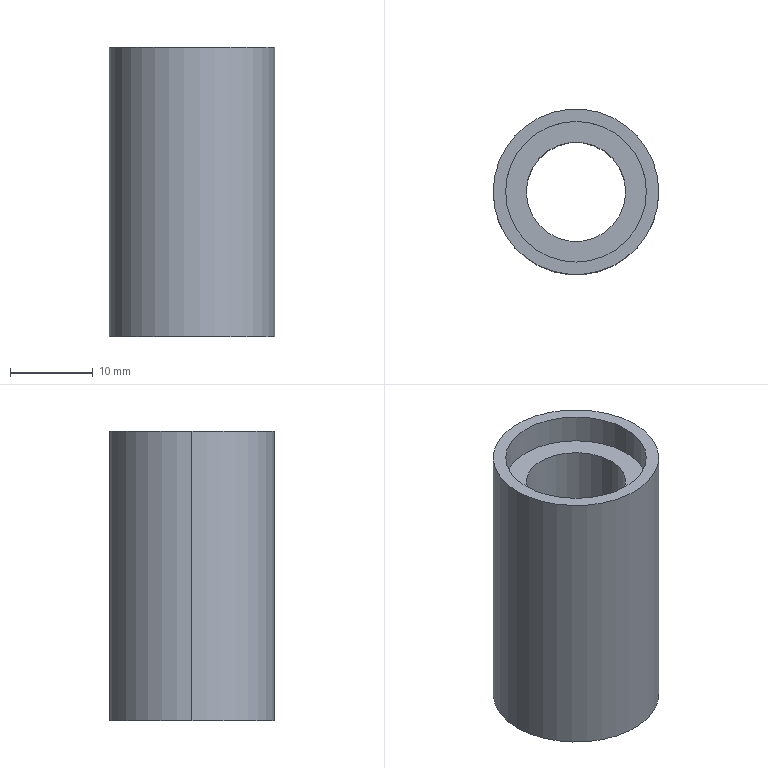Part | STEP file | 1 solid | 11 faces | box 20 x 20 x 35 mm | volume 6555 mm3 | cylinder 6 | plane 3 | cone 2 | commonest cylinder face diameters 12 x2 17 x2 20 x2
STEP:
#1=CARTESIAN_POINT('',(0.,0.,0.));
#2=DIRECTION('',(0.,0.,1.));
#3=DIRECTION('',(1.,0.,0.));
#4=AXIS2_PLACEMENT_3D('',#1,#2,#3);
#5=CARTESIAN_POINT('',(10.,0.,0.));
#6=VERTEX_POINT('',#5);
#7=CARTESIAN_POINT('',(-10.,0.,0.));
#8=VERTEX_POINT('',#7);
#9=CARTESIAN_POINT('',(0.,0.,0.));
#10=DIRECTION('',(0.,0.,1.));
#11=DIRECTION('',(1.,0.,0.));
#12=AXIS2_PLACEMENT_3D('',#9,#10,#11);
#13=CIRCLE('',#12,10.);
#14=CARTESIAN_POINT('',(0.,0.,0.));
#15=DIRECTION('',(0.,0.,1.));
#16=DIRECTION('',(1.,0.,0.));
#17=AXIS2_PLACEMENT_3D('',#14,#15,#16);
#18=CYLINDRICAL_SURFACE('',#17,10.);
#19=CARTESIAN_POINT('',(0.,0.));
#20=DIRECTION('',(1.,0.));
#21=VECTOR('',#20,1.);
#22=LINE('',#19,#21);
#23=(GEOMETRIC_REPRESENTATION_CONTEXT(2)PARAMETRIC_REPRESENTATION_CONTEXT()REPRESENTATION_CONTEXT('',''));
#24=DEFINITIONAL_REPRESENTATION('',(#22),#23);
#25=PCURVE('',#18,#24);
#26=CARTESIAN_POINT('',(0.,0.,0.));
#27=DIRECTION('',(0.,0.,-1.));
#28=DIRECTION('',(-1.,0.,0.));
#29=AXIS2_PLACEMENT_3D('',#26,#27,#28);
#30=PLANE('',#29);
#31=CARTESIAN_POINT('',(-10.,0.));
#32=CARTESIAN_POINT('',(-10.,17.321));
#33=CARTESIAN_POINT('',(5.,8.66));
#34=CARTESIAN_POINT('',(20.,0.));
#35=CARTESIAN_POINT('',(5.,-8.66));
#36=CARTESIAN_POINT('',(-10.,-17.321));
#37=CARTESIAN_POINT('',(-10.,0.));
#38=(BOUNDED_CURVE()B_SPLINE_CURVE(2,(#31,#32,#33,#34,#35,#36,#37),.UNSPECIFIED.,.T.,.F.)B_SPLINE_CURVE_WITH_KNOTS((1,2,2,2,2,1),(-2.094,0.,2.094,4.189,6.283,8.378),.UNSPECIFIED.)CURVE()GEOMETRIC_REPRESENTATION_ITEM()RATIONAL_B_SPLINE_CURVE((1.,0.5,1.,0.5,1.,0.5,1.))REPRESENTATION_ITEM(''));
#39=(GEOMETRIC_REPRESENTATION_CONTEXT(2)PARAMETRIC_REPRESENTATION_CONTEXT()REPRESENTATION_CONTEXT('',''));
#40=DEFINITIONAL_REPRESENTATION('',(#38),#39);
#41=PCURVE('',#30,#40);
#42=SURFACE_CURVE('',#13,(#25,#41),.PCURVE_S1.);
#43=EDGE_CURVE('',#6,#8,#42,.T.);
#44=ORIENTED_EDGE('',*,*,#43,.T.);
#45=CARTESIAN_POINT('',(-10.,0.,35.));
#46=VERTEX_POINT('',#45);
#47=CARTESIAN_POINT('',(-10.,0.,0.));
#48=DIRECTION('',(0.,0.,1.));
#49=VECTOR('',#48,1.);
#50=LINE('',#47,#49);
#51=CARTESIAN_POINT('',(3.142,0.));
#52=DIRECTION('',(0.,1.));
#53=VECTOR('',#52,1.);
#54=LINE('',#51,#53);
#55=(GEOMETRIC_REPRESENTATION_CONTEXT(2)PARAMETRIC_REPRESENTATION_CONTEXT()REPRESENTATION_CONTEXT('',''));
#56=DEFINITIONAL_REPRESENTATION('',(#54),#55);
#57=PCURVE('',#18,#56);
#58=CARTESIAN_POINT('',(0.,0.,0.));
#59=DIRECTION('',(0.,0.,1.));
#60=DIRECTION('',(1.,0.,0.));
#61=AXIS2_PLACEMENT_3D('',#58,#59,#60);
#62=CYLINDRICAL_SURFACE('',#61,10.);
#63=CARTESIAN_POINT('',(3.142,0.));
#64=DIRECTION('',(0.,1.));
#65=VECTOR('',#64,1.);
#66=LINE('',#63,#65);
#67=(GEOMETRIC_REPRESENTATION_CONTEXT(2)PARAMETRIC_REPRESENTATION_CONTEXT()REPRESENTATION_CONTEXT('',''));
#68=DEFINITIONAL_REPRESENTATION('',(#66),#67);
#69=PCURVE('',#62,#68);
#70=SURFACE_CURVE('',#50,(#57,#69),.PCURVE_S1.);
#71=EDGE_CURVE('',#8,#46,#70,.T.);
#72=ORIENTED_EDGE('',*,*,#71,.T.);
#73=CARTESIAN_POINT('',(10.,0.,35.));
#74=VERTEX_POINT('',#73);
#75=CARTESIAN_POINT('',(0.,0.,35.));
#76=DIRECTION('',(0.,0.,-1.));
#77=DIRECTION('',(1.,0.,0.));
#78=AXIS2_PLACEMENT_3D('',#75,#76,#77);
#79=CIRCLE('',#78,10.);
#80=CARTESIAN_POINT('',(6.283,35.));
#81=DIRECTION('',(-1.,0.));
#82=VECTOR('',#81,1.);
#83=LINE('',#80,#82);
#84=(GEOMETRIC_REPRESENTATION_CONTEXT(2)PARAMETRIC_REPRESENTATION_CONTEXT()REPRESENTATION_CONTEXT('',''));
#85=DEFINITIONAL_REPRESENTATION('',(#83),#84);
#86=PCURVE('',#18,#85);
#87=CARTESIAN_POINT('',(0.,0.,35.));
#88=DIRECTION('',(0.,0.,-1.));
#89=DIRECTION('',(-1.,0.,0.));
#90=AXIS2_PLACEMENT_3D('',#87,#88,#89);
#91=PLANE('',#90);
#92=CARTESIAN_POINT('',(0.,0.));
#93=DIRECTION('',(-1.,0.));
#94=AXIS2_PLACEMENT_2D('',#92,#93);
#95=CIRCLE('',#94,10.);
#96=(GEOMETRIC_REPRESENTATION_CONTEXT(2)PARAMETRIC_REPRESENTATION_CONTEXT()REPRESENTATION_CONTEXT('',''));
#97=DEFINITIONAL_REPRESENTATION('',(#95),#96);
#98=PCURVE('',#91,#97);
#99=SURFACE_CURVE('',#79,(#86,#98),.PCURVE_S1.);
#100=EDGE_CURVE('',#46,#74,#99,.T.);
#101=ORIENTED_EDGE('',*,*,#100,.T.);
#102=CARTESIAN_POINT('',(10.,0.,0.));
#103=DIRECTION('',(0.,0.,1.));
#104=VECTOR('',#103,1.);
#105=LINE('',#102,#104);
#106=CARTESIAN_POINT('',(0.,0.));
#107=DIRECTION('',(0.,1.));
#108=VECTOR('',#107,1.);
#109=LINE('',#106,#108);
#110=(GEOMETRIC_REPRESENTATION_CONTEXT(2)PARAMETRIC_REPRESENTATION_CONTEXT()REPRESENTATION_CONTEXT('',''));
#111=DEFINITIONAL_REPRESENTATION('',(#109),#110);
#112=PCURVE('',#18,#111);
#113=CARTESIAN_POINT('',(6.283,0.));
#114=DIRECTION('',(0.,1.));
#115=VECTOR('',#114,1.);
#116=LINE('',#113,#115);
#117=(GEOMETRIC_REPRESENTATION_CONTEXT(2)PARAMETRIC_REPRESENTATION_CONTEXT()REPRESENTATION_CONTEXT('',''));
#118=DEFINITIONAL_REPRESENTATION('',(#116),#117);
#119=PCURVE('',#62,#118);
#120=SURFACE_CURVE('',#105,(#112,#119),.PCURVE_S1.);
#121=EDGE_CURVE('',#6,#74,#120,.T.);
#122=ORIENTED_EDGE('',*,*,#121,.F.);
#123=EDGE_LOOP('',(#44,#72,#101,#122));
#124=FACE_BOUND('',#123,.T.);
#125=ADVANCED_FACE('',(#124),#18,.T.);
#126=CARTESIAN_POINT('',(-6.,0.,2.));
#127=VERTEX_POINT('',#126);
#128=CARTESIAN_POINT('',(-8.,0.,-0.000000001));
#129=VERTEX_POINT('',#128);
#130=CARTESIAN_POINT('',(-8.,0.,-0.000000001));
#131=DIRECTION('',(-0.7071,0.,-0.7071));
#132=VECTOR('',#131,1.);
#133=LINE('',#130,#132);
#134=CARTESIAN_POINT('',(0.,0.,-0.000000001));
#135=DIRECTION('',(0.,0.,-1.));
#136=DIRECTION('',(-1.,0.,0.));
#137=AXIS2_PLACEMENT_3D('',#134,#135,#136);
#138=CONICAL_SURFACE('',#137,8.,0.7854);
#139=CARTESIAN_POINT('',(6.283,0.));
#140=DIRECTION('',(0.,1.));
#141=VECTOR('',#140,1.);
#142=LINE('',#139,#141);
#143=(GEOMETRIC_REPRESENTATION_CONTEXT(2)PARAMETRIC_REPRESENTATION_CONTEXT()REPRESENTATION_CONTEXT('',''));
#144=DEFINITIONAL_REPRESENTATION('',(#142),#143);
#145=PCURVE('',#138,#144);
#146=CARTESIAN_POINT('',(0.,0.,-0.000000001));
#147=DIRECTION('',(0.,0.,-1.));
#148=DIRECTION('',(-1.,0.,0.));
#149=AXIS2_PLACEMENT_3D('',#146,#147,#148);
#150=CONICAL_SURFACE('',#149,8.,0.7854);
#151=CARTESIAN_POINT('',(0.,0.));
#152=DIRECTION('',(0.,1.));
#153=VECTOR('',#152,1.);
#154=LINE('',#151,#153);
#155=(GEOMETRIC_REPRESENTATION_CONTEXT(2)PARAMETRIC_REPRESENTATION_CONTEXT()REPRESENTATION_CONTEXT('',''));
#156=DEFINITIONAL_REPRESENTATION('',(#154),#155);
#157=PCURVE('',#150,#156);
#158=SURFACE_CURVE('',#133,(#145,#157),.PCURVE_S1.);
#159=EDGE_CURVE('',#127,#129,#158,.T.);
#160=ORIENTED_EDGE('',*,*,#159,.T.);
#161=CARTESIAN_POINT('',(8.,0.,-0.000000001));
#162=VERTEX_POINT('',#161);
#163=CARTESIAN_POINT('',(0.,0.,-0.000000001));
#164=DIRECTION('',(0.,0.,1.));
#165=DIRECTION('',(-1.,0.,0.));
#166=AXIS2_PLACEMENT_3D('',#163,#164,#165);
#167=CIRCLE('',#166,8.);
#168=CARTESIAN_POINT('',(6.283,0.));
#169=DIRECTION('',(-1.,0.));
#170=VECTOR('',#169,1.);
#171=LINE('',#168,#170);
#172=(GEOMETRIC_REPRESENTATION_CONTEXT(2)PARAMETRIC_REPRESENTATION_CONTEXT()REPRESENTATION_CONTEXT('',''));
#173=DEFINITIONAL_REPRESENTATION('',(#171),#172);
#174=PCURVE('',#138,#173);
#175=CARTESIAN_POINT('',(8.,0.));
#176=CARTESIAN_POINT('',(8.,-13.856));
#177=CARTESIAN_POINT('',(-4.,-6.928));
#178=CARTESIAN_POINT('',(-16.,0.));
#179=CARTESIAN_POINT('',(-4.,6.928));
#180=CARTESIAN_POINT('',(8.,13.856));
#181=CARTESIAN_POINT('',(8.,0.));
#182=(BOUNDED_CURVE()B_SPLINE_CURVE(2,(#175,#176,#177,#178,#179,#180,#181),.UNSPECIFIED.,.T.,.F.)B_SPLINE_CURVE_WITH_KNOTS((1,2,2,2,2,1),(-2.094,0.,2.094,4.189,6.283,8.378),.UNSPECIFIED.)CURVE()GEOMETRIC_REPRESENTATION_ITEM()RATIONAL_B_SPLINE_CURVE((1.,0.5,1.,0.5,1.,0.5,1.))REPRESENTATION_ITEM(''));
#183=(GEOMETRIC_REPRESENTATION_CONTEXT(2)PARAMETRIC_REPRESENTATION_CONTEXT()REPRESENTATION_CONTEXT('',''));
#184=DEFINITIONAL_REPRESENTATION('',(#182),#183);
#185=PCURVE('',#30,#184);
#186=SURFACE_CURVE('',#167,(#174,#185),.PCURVE_S1.);
#187=EDGE_CURVE('',#129,#162,#186,.T.);
#188=ORIENTED_EDGE('',*,*,#187,.T.);
#189=CARTESIAN_POINT('',(6.,0.,2.));
#190=VERTEX_POINT('',#189);
#191=CARTESIAN_POINT('',(8.,0.,-0.000000001));
#192=DIRECTION('',(0.7071,0.,-0.7071));
#193=VECTOR('',#192,1.);
#194=LINE('',#191,#193);
#195=CARTESIAN_POINT('',(3.142,0.));
#196=DIRECTION('',(0.,1.));
#197=VECTOR('',#196,1.);
#198=LINE('',#195,#197);
#199=(GEOMETRIC_REPRESENTATION_CONTEXT(2)PARAMETRIC_REPRESENTATION_CONTEXT()REPRESENTATION_CONTEXT('',''));
#200=DEFINITIONAL_REPRESENTATION('',(#198),#199);
#201=PCURVE('',#138,#200);
#202=CARTESIAN_POINT('',(3.142,0.));
#203=DIRECTION('',(0.,1.));
#204=VECTOR('',#203,1.);
#205=LINE('',#202,#204);
#206=(GEOMETRIC_REPRESENTATION_CONTEXT(2)PARAMETRIC_REPRESENTATION_CONTEXT()REPRESENTATION_CONTEXT('',''));
#207=DEFINITIONAL_REPRESENTATION('',(#205),#206);
#208=PCURVE('',#150,#207);
#209=SURFACE_CURVE('',#194,(#201,#208),.PCURVE_S1.);
#210=EDGE_CURVE('',#190,#162,#209,.T.);
#211=ORIENTED_EDGE('',*,*,#210,.F.);
#212=CARTESIAN_POINT('',(0.,0.,2.));
#213=DIRECTION('',(0.,0.,-1.));
#214=DIRECTION('',(1.,0.,0.));
#215=AXIS2_PLACEMENT_3D('',#212,#213,#214);
#216=CIRCLE('',#215,6.);
#217=CARTESIAN_POINT('',(3.142,-2.));
#218=DIRECTION('',(1.,0.));
#219=VECTOR('',#218,1.);
#220=LINE('',#217,#219);
#221=(GEOMETRIC_REPRESENTATION_CONTEXT(2)PARAMETRIC_REPRESENTATION_CONTEXT()REPRESENTATION_CONTEXT('',''));
#222=DEFINITIONAL_REPRESENTATION('',(#220),#221);
#223=PCURVE('',#138,#222);
#224=CARTESIAN_POINT('',(0.,0.,0.));
#225=DIRECTION('',(0.,0.,1.));
#226=DIRECTION('',(1.,0.,0.));
#227=AXIS2_PLACEMENT_3D('',#224,#225,#226);
#228=CYLINDRICAL_SURFACE('',#227,6.);
#229=CARTESIAN_POINT('',(6.283,2.));
#230=DIRECTION('',(-1.,0.));
#231=VECTOR('',#230,1.);
#232=LINE('',#229,#231);
#233=(GEOMETRIC_REPRESENTATION_CONTEXT(2)PARAMETRIC_REPRESENTATION_CONTEXT()REPRESENTATION_CONTEXT('',''));
#234=DEFINITIONAL_REPRESENTATION('',(#232),#233);
#235=PCURVE('',#228,#234);
#236=SURFACE_CURVE('',#216,(#223,#235),.PCURVE_S1.);
#237=EDGE_CURVE('',#190,#127,#236,.T.);
#238=ORIENTED_EDGE('',*,*,#237,.T.);
#239=EDGE_LOOP('',(#160,#188,#211,#238));
#240=FACE_BOUND('',#239,.F.);
#241=ADVANCED_FACE('',(#240),#138,.F.);
#242=CARTESIAN_POINT('',(-8.5,0.,35.));
#243=VERTEX_POINT('',#242);
#244=CARTESIAN_POINT('',(-8.5,0.,31.5));
#245=VERTEX_POINT('',#244);
#246=CARTESIAN_POINT('',(-8.5,0.,35.));
#247=DIRECTION('',(0.,0.,-1.));
#248=VECTOR('',#247,1.);
#249=LINE('',#246,#248);
#250=CARTESIAN_POINT('',(0.,0.,35.));
#251=DIRECTION('',(0.,0.,-1.));
#252=DIRECTION('',(-1.,0.,0.));
#253=AXIS2_PLACEMENT_3D('',#250,#251,#252);
#254=CYLINDRICAL_SURFACE('',#253,8.5);
#255=CARTESIAN_POINT('',(6.283,0.));
#256=DIRECTION('',(0.,1.));
#257=VECTOR('',#256,1.);
#258=LINE('',#255,#257);
#259=(GEOMETRIC_REPRESENTATION_CONTEXT(2)PARAMETRIC_REPRESENTATION_CONTEXT()REPRESENTATION_CONTEXT('',''));
#260=DEFINITIONAL_REPRESENTATION('',(#258),#259);
#261=PCURVE('',#254,#260);
#262=CARTESIAN_POINT('',(0.,0.,35.));
#263=DIRECTION('',(0.,0.,-1.));
#264=DIRECTION('',(-1.,0.,0.));
#265=AXIS2_PLACEMENT_3D('',#262,#263,#264);
#266=CYLINDRICAL_SURFACE('',#265,8.5);
#267=CARTESIAN_POINT('',(0.,0.));
#268=DIRECTION('',(0.,1.));
#269=VECTOR('',#268,1.);
#270=LINE('',#267,#269);
#271=(GEOMETRIC_REPRESENTATION_CONTEXT(2)PARAMETRIC_REPRESENTATION_CONTEXT()REPRESENTATION_CONTEXT('',''));
#272=DEFINITIONAL_REPRESENTATION('',(#270),#271);
#273=PCURVE('',#266,#272);
#274=SURFACE_CURVE('',#249,(#261,#273),.PCURVE_S1.);
#275=EDGE_CURVE('',#243,#245,#274,.T.);
#276=ORIENTED_EDGE('',*,*,#275,.T.);
#277=CARTESIAN_POINT('',(8.5,0.,31.5));
#278=VERTEX_POINT('',#277);
#279=CARTESIAN_POINT('',(0.,0.,31.5));
#280=DIRECTION('',(0.,0.,1.));
#281=DIRECTION('',(-1.,0.,0.));
#282=AXIS2_PLACEMENT_3D('',#279,#280,#281);
#283=CIRCLE('',#282,8.5);
#284=CARTESIAN_POINT('',(6.283,3.5));
#285=DIRECTION('',(-1.,0.));
#286=VECTOR('',#285,1.);
#287=LINE('',#284,#286);
#288=(GEOMETRIC_REPRESENTATION_CONTEXT(2)PARAMETRIC_REPRESENTATION_CONTEXT()REPRESENTATION_CONTEXT('',''));
#289=DEFINITIONAL_REPRESENTATION('',(#287),#288);
#290=PCURVE('',#254,#289);
#291=CARTESIAN_POINT('',(0.,0.,31.5));
#292=DIRECTION('',(0.,0.,-1.));
#293=DIRECTION('',(-1.,0.,0.));
#294=AXIS2_PLACEMENT_3D('',#291,#292,#293);
#295=PLANE('',#294);
#296=CARTESIAN_POINT('',(8.5,0.));
#297=CARTESIAN_POINT('',(8.5,-14.722));
#298=CARTESIAN_POINT('',(-4.25,-7.361));
#299=CARTESIAN_POINT('',(-17.,0.));
#300=CARTESIAN_POINT('',(-4.25,7.361));
#301=CARTESIAN_POINT('',(8.5,14.722));
#302=CARTESIAN_POINT('',(8.5,0.));
#303=(BOUNDED_CURVE()B_SPLINE_CURVE(2,(#296,#297,#298,#299,#300,#301,#302),.UNSPECIFIED.,.T.,.F.)B_SPLINE_CURVE_WITH_KNOTS((1,2,2,2,2,1),(-2.094,0.,2.094,4.189,6.283,8.378),.UNSPECIFIED.)CURVE()GEOMETRIC_REPRESENTATION_ITEM()RATIONAL_B_SPLINE_CURVE((1.,0.5,1.,0.5,1.,0.5,1.))REPRESENTATION_ITEM(''));
#304=(GEOMETRIC_REPRESENTATION_CONTEXT(2)PARAMETRIC_REPRESENTATION_CONTEXT()REPRESENTATION_CONTEXT('',''));
#305=DEFINITIONAL_REPRESENTATION('',(#303),#304);
#306=PCURVE('',#295,#305);
#307=SURFACE_CURVE('',#283,(#290,#306),.PCURVE_S1.);
#308=EDGE_CURVE('',#245,#278,#307,.T.);
#309=ORIENTED_EDGE('',*,*,#308,.T.);
#310=CARTESIAN_POINT('',(8.5,0.,35.));
#311=VERTEX_POINT('',#310);
#312=CARTESIAN_POINT('',(8.5,0.,35.));
#313=DIRECTION('',(0.,0.,-1.));
#314=VECTOR('',#313,1.);
#315=LINE('',#312,#314);
#316=CARTESIAN_POINT('',(3.142,0.));
#317=DIRECTION('',(0.,1.));
#318=VECTOR('',#317,1.);
#319=LINE('',#316,#318);
#320=(GEOMETRIC_REPRESENTATION_CONTEXT(2)PARAMETRIC_REPRESENTATION_CONTEXT()REPRESENTATION_CONTEXT('',''));
#321=DEFINITIONAL_REPRESENTATION('',(#319),#320);
#322=PCURVE('',#254,#321);
#323=CARTESIAN_POINT('',(3.142,0.));
#324=DIRECTION('',(0.,1.));
#325=VECTOR('',#324,1.);
#326=LINE('',#323,#325);
#327=(GEOMETRIC_REPRESENTATION_CONTEXT(2)PARAMETRIC_REPRESENTATION_CONTEXT()REPRESENTATION_CONTEXT('',''));
#328=DEFINITIONAL_REPRESENTATION('',(#326),#327);
#329=PCURVE('',#266,#328);
#330=SURFACE_CURVE('',#315,(#322,#329),.PCURVE_S1.);
#331=EDGE_CURVE('',#311,#278,#330,.T.);
#332=ORIENTED_EDGE('',*,*,#331,.F.);
#333=CARTESIAN_POINT('',(0.,0.,35.));
#334=DIRECTION('',(0.,0.,1.));
#335=DIRECTION('',(-1.,0.,0.));
#336=AXIS2_PLACEMENT_3D('',#333,#334,#335);
#337=CIRCLE('',#336,8.5);
#338=CARTESIAN_POINT('',(6.283,0.));
#339=DIRECTION('',(-1.,0.));
#340=VECTOR('',#339,1.);
#341=LINE('',#338,#340);
#342=(GEOMETRIC_REPRESENTATION_CONTEXT(2)PARAMETRIC_REPRESENTATION_CONTEXT()REPRESENTATION_CONTEXT('',''));
#343=DEFINITIONAL_REPRESENTATION('',(#341),#342);
#344=PCURVE('',#254,#343);
#345=CARTESIAN_POINT('',(8.5,0.));
#346=CARTESIAN_POINT('',(8.5,-14.722));
#347=CARTESIAN_POINT('',(-4.25,-7.361));
#348=CARTESIAN_POINT('',(-17.,0.));
#349=CARTESIAN_POINT('',(-4.25,7.361));
#350=CARTESIAN_POINT('',(8.5,14.722));
#351=CARTESIAN_POINT('',(8.5,0.));
#352=(BOUNDED_CURVE()B_SPLINE_CURVE(2,(#345,#346,#347,#348,#349,#350,#351),.UNSPECIFIED.,.T.,.F.)B_SPLINE_CURVE_WITH_KNOTS((1,2,2,2,2,1),(-2.094,0.,2.094,4.189,6.283,8.378),.UNSPECIFIED.)CURVE()GEOMETRIC_REPRESENTATION_ITEM()RATIONAL_B_SPLINE_CURVE((1.,0.5,1.,0.5,1.,0.5,1.))REPRESENTATION_ITEM(''));
#353=(GEOMETRIC_REPRESENTATION_CONTEXT(2)PARAMETRIC_REPRESENTATION_CONTEXT()REPRESENTATION_CONTEXT('',''));
#354=DEFINITIONAL_REPRESENTATION('',(#352),#353);
#355=PCURVE('',#91,#354);
#356=SURFACE_CURVE('',#337,(#344,#355),.PCURVE_S1.);
#357=EDGE_CURVE('',#243,#311,#356,.T.);
#358=ORIENTED_EDGE('',*,*,#357,.F.);
#359=EDGE_LOOP('',(#276,#309,#332,#358));
#360=FACE_BOUND('',#359,.F.);
#361=ADVANCED_FACE('',(#360),#254,.F.);
#362=CARTESIAN_POINT('',(6.,0.,31.5));
#363=VERTEX_POINT('',#362);
#364=CARTESIAN_POINT('',(6.,0.,0.));
#365=DIRECTION('',(0.,0.,1.));
#366=VECTOR('',#365,1.);
#367=LINE('',#364,#366);
#368=CARTESIAN_POINT('',(6.283,0.));
#369=DIRECTION('',(0.,1.));
#370=VECTOR('',#369,1.);
#371=LINE('',#368,#370);
#372=(GEOMETRIC_REPRESENTATION_CONTEXT(2)PARAMETRIC_REPRESENTATION_CONTEXT()REPRESENTATION_CONTEXT('',''));
#373=DEFINITIONAL_REPRESENTATION('',(#371),#372);
#374=PCURVE('',#228,#373);
#375=CARTESIAN_POINT('',(0.,0.,0.));
#376=DIRECTION('',(0.,0.,1.));
#377=DIRECTION('',(1.,0.,0.));
#378=AXIS2_PLACEMENT_3D('',#375,#376,#377);
#379=CYLINDRICAL_SURFACE('',#378,6.);
#380=CARTESIAN_POINT('',(0.,0.));
#381=DIRECTION('',(0.,1.));
#382=VECTOR('',#381,1.);
#383=LINE('',#380,#382);
#384=(GEOMETRIC_REPRESENTATION_CONTEXT(2)PARAMETRIC_REPRESENTATION_CONTEXT()REPRESENTATION_CONTEXT('',''));
#385=DEFINITIONAL_REPRESENTATION('',(#383),#384);
#386=PCURVE('',#379,#385);
#387=SURFACE_CURVE('',#367,(#374,#386),.PCURVE_S1.);
#388=EDGE_CURVE('',#190,#363,#387,.T.);
#389=ORIENTED_EDGE('',*,*,#388,.T.);
#390=CARTESIAN_POINT('',(-6.,0.,31.5));
#391=VERTEX_POINT('',#390);
#392=CARTESIAN_POINT('',(0.,0.,31.5));
#393=DIRECTION('',(0.,0.,-1.));
#394=DIRECTION('',(1.,0.,0.));
#395=AXIS2_PLACEMENT_3D('',#392,#393,#394);
#396=CIRCLE('',#395,6.);
#397=CARTESIAN_POINT('',(6.283,31.5));
#398=DIRECTION('',(-1.,0.));
#399=VECTOR('',#398,1.);
#400=LINE('',#397,#399);
#401=(GEOMETRIC_REPRESENTATION_CONTEXT(2)PARAMETRIC_REPRESENTATION_CONTEXT()REPRESENTATION_CONTEXT('',''));
#402=DEFINITIONAL_REPRESENTATION('',(#400),#401);
#403=PCURVE('',#228,#402);
#404=CARTESIAN_POINT('',(0.,0.));
#405=DIRECTION('',(-1.,0.));
#406=AXIS2_PLACEMENT_2D('',#404,#405);
#407=CIRCLE('',#406,6.);
#408=(GEOMETRIC_REPRESENTATION_CONTEXT(2)PARAMETRIC_REPRESENTATION_CONTEXT()REPRESENTATION_CONTEXT('',''));
#409=DEFINITIONAL_REPRESENTATION('',(#407),#408);
#410=PCURVE('',#295,#409);
#411=SURFACE_CURVE('',#396,(#403,#410),.PCURVE_S1.);
#412=EDGE_CURVE('',#363,#391,#411,.T.);
#413=ORIENTED_EDGE('',*,*,#412,.T.);
#414=CARTESIAN_POINT('',(-6.,0.,0.));
#415=DIRECTION('',(0.,0.,1.));
#416=VECTOR('',#415,1.);
#417=LINE('',#414,#416);
#418=CARTESIAN_POINT('',(3.142,0.));
#419=DIRECTION('',(0.,1.));
#420=VECTOR('',#419,1.);
#421=LINE('',#418,#420);
#422=(GEOMETRIC_REPRESENTATION_CONTEXT(2)PARAMETRIC_REPRESENTATION_CONTEXT()REPRESENTATION_CONTEXT('',''));
#423=DEFINITIONAL_REPRESENTATION('',(#421),#422);
#424=PCURVE('',#228,#423);
#425=CARTESIAN_POINT('',(3.142,0.));
#426=DIRECTION('',(0.,1.));
#427=VECTOR('',#426,1.);
#428=LINE('',#425,#427);
#429=(GEOMETRIC_REPRESENTATION_CONTEXT(2)PARAMETRIC_REPRESENTATION_CONTEXT()REPRESENTATION_CONTEXT('',''));
#430=DEFINITIONAL_REPRESENTATION('',(#428),#429);
#431=PCURVE('',#379,#430);
#432=SURFACE_CURVE('',#417,(#424,#431),.PCURVE_S1.);
#433=EDGE_CURVE('',#127,#391,#432,.T.);
#434=ORIENTED_EDGE('',*,*,#433,.F.);
#435=ORIENTED_EDGE('',*,*,#237,.F.);
#436=EDGE_LOOP('',(#389,#413,#434,#435));
#437=FACE_BOUND('',#436,.F.);
#438=ADVANCED_FACE('',(#437),#228,.F.);
#439=ORIENTED_EDGE('',*,*,#71,.F.);
#440=CARTESIAN_POINT('',(0.,0.,0.));
#441=DIRECTION('',(0.,0.,1.));
#442=DIRECTION('',(1.,0.,0.));
#443=AXIS2_PLACEMENT_3D('',#440,#441,#442);
#444=CIRCLE('',#443,10.);
#445=CARTESIAN_POINT('',(0.,0.));
#446=DIRECTION('',(1.,0.));
#447=VECTOR('',#446,1.);
#448=LINE('',#445,#447);
#449=(GEOMETRIC_REPRESENTATION_CONTEXT(2)PARAMETRIC_REPRESENTATION_CONTEXT()REPRESENTATION_CONTEXT('',''));
#450=DEFINITIONAL_REPRESENTATION('',(#448),#449);
#451=PCURVE('',#62,#450);
#452=CARTESIAN_POINT('',(-10.,0.));
#453=CARTESIAN_POINT('',(-10.,17.321));
#454=CARTESIAN_POINT('',(5.,8.66));
#455=CARTESIAN_POINT('',(20.,0.));
#456=CARTESIAN_POINT('',(5.,-8.66));
#457=CARTESIAN_POINT('',(-10.,-17.321));
#458=CARTESIAN_POINT('',(-10.,0.));
#459=(BOUNDED_CURVE()B_SPLINE_CURVE(2,(#452,#453,#454,#455,#456,#457,#458),.UNSPECIFIED.,.T.,.F.)B_SPLINE_CURVE_WITH_KNOTS((1,2,2,2,2,1),(-2.094,0.,2.094,4.189,6.283,8.378),.UNSPECIFIED.)CURVE()GEOMETRIC_REPRESENTATION_ITEM()RATIONAL_B_SPLINE_CURVE((1.,0.5,1.,0.5,1.,0.5,1.))REPRESENTATION_ITEM(''));
#460=(GEOMETRIC_REPRESENTATION_CONTEXT(2)PARAMETRIC_REPRESENTATION_CONTEXT()REPRESENTATION_CONTEXT('',''));
#461=DEFINITIONAL_REPRESENTATION('',(#459),#460);
#462=PCURVE('',#30,#461);
#463=SURFACE_CURVE('',#444,(#451,#462),.PCURVE_S1.);
#464=EDGE_CURVE('',#8,#6,#463,.T.);
#465=ORIENTED_EDGE('',*,*,#464,.T.);
#466=ORIENTED_EDGE('',*,*,#121,.T.);
#467=CARTESIAN_POINT('',(0.,0.,35.));
#468=DIRECTION('',(0.,0.,-1.));
#469=DIRECTION('',(1.,0.,0.));
#470=AXIS2_PLACEMENT_3D('',#467,#468,#469);
#471=CIRCLE('',#470,10.);
#472=CARTESIAN_POINT('',(6.283,35.));
#473=DIRECTION('',(-1.,0.));
#474=VECTOR('',#473,1.);
#475=LINE('',#472,#474);
#476=(GEOMETRIC_REPRESENTATION_CONTEXT(2)PARAMETRIC_REPRESENTATION_CONTEXT()REPRESENTATION_CONTEXT('',''));
#477=DEFINITIONAL_REPRESENTATION('',(#475),#476);
#478=PCURVE('',#62,#477);
#479=CARTESIAN_POINT('',(0.,0.));
#480=DIRECTION('',(-1.,0.));
#481=AXIS2_PLACEMENT_2D('',#479,#480);
#482=CIRCLE('',#481,10.);
#483=(GEOMETRIC_REPRESENTATION_CONTEXT(2)PARAMETRIC_REPRESENTATION_CONTEXT()REPRESENTATION_CONTEXT('',''));
#484=DEFINITIONAL_REPRESENTATION('',(#482),#483);
#485=PCURVE('',#91,#484);
#486=SURFACE_CURVE('',#471,(#478,#485),.PCURVE_S1.);
#487=EDGE_CURVE('',#74,#46,#486,.T.);
#488=ORIENTED_EDGE('',*,*,#487,.T.);
#489=EDGE_LOOP('',(#439,#465,#466,#488));
#490=FACE_BOUND('',#489,.T.);
#491=ADVANCED_FACE('',(#490),#62,.T.);
#492=ORIENTED_EDGE('',*,*,#187,.T.);
#493=CARTESIAN_POINT('',(0.,0.,-0.000000001));
#494=DIRECTION('',(0.,0.,1.));
#495=DIRECTION('',(-1.,0.,0.));
#496=AXIS2_PLACEMENT_3D('',#493,#494,#495);
#497=CIRCLE('',#496,8.);
#498=CARTESIAN_POINT('',(8.,0.));
#499=CARTESIAN_POINT('',(8.,-13.856));
#500=CARTESIAN_POINT('',(-4.,-6.928));
#501=CARTESIAN_POINT('',(-16.,0.));
#502=CARTESIAN_POINT('',(-4.,6.928));
#503=CARTESIAN_POINT('',(8.,13.856));
#504=CARTESIAN_POINT('',(8.,0.));
#505=(BOUNDED_CURVE()B_SPLINE_CURVE(2,(#498,#499,#500,#501,#502,#503,#504),.UNSPECIFIED.,.T.,.F.)B_SPLINE_CURVE_WITH_KNOTS((1,2,2,2,2,1),(-2.094,0.,2.094,4.189,6.283,8.378),.UNSPECIFIED.)CURVE()GEOMETRIC_REPRESENTATION_ITEM()RATIONAL_B_SPLINE_CURVE((1.,0.5,1.,0.5,1.,0.5,1.))REPRESENTATION_ITEM(''));
#506=(GEOMETRIC_REPRESENTATION_CONTEXT(2)PARAMETRIC_REPRESENTATION_CONTEXT()REPRESENTATION_CONTEXT('',''));
#507=DEFINITIONAL_REPRESENTATION('',(#505),#506);
#508=PCURVE('',#30,#507);
#509=CARTESIAN_POINT('',(6.283,0.));
#510=DIRECTION('',(-1.,0.));
#511=VECTOR('',#510,1.);
#512=LINE('',#509,#511);
#513=(GEOMETRIC_REPRESENTATION_CONTEXT(2)PARAMETRIC_REPRESENTATION_CONTEXT()REPRESENTATION_CONTEXT('',''));
#514=DEFINITIONAL_REPRESENTATION('',(#512),#513);
#515=PCURVE('',#150,#514);
#516=SURFACE_CURVE('',#497,(#508,#515),.PCURVE_S1.);
#517=EDGE_CURVE('',#162,#129,#516,.T.);
#518=ORIENTED_EDGE('',*,*,#517,.T.);
#519=EDGE_LOOP('',(#492,#518));
#520=FACE_BOUND('',#519,.T.);
#521=ORIENTED_EDGE('',*,*,#43,.F.);
#522=ORIENTED_EDGE('',*,*,#464,.F.);
#523=EDGE_LOOP('',(#521,#522));
#524=FACE_BOUND('',#523,.T.);
#525=ADVANCED_FACE('',(#520,#524),#30,.T.);
#526=ORIENTED_EDGE('',*,*,#357,.F.);
#527=CARTESIAN_POINT('',(0.,0.,35.));
#528=DIRECTION('',(0.,0.,1.));
#529=DIRECTION('',(-1.,0.,0.));
#530=AXIS2_PLACEMENT_3D('',#527,#528,#529);
#531=CIRCLE('',#530,8.5);
#532=CARTESIAN_POINT('',(8.5,0.));
#533=CARTESIAN_POINT('',(8.5,-14.722));
#534=CARTESIAN_POINT('',(-4.25,-7.361));
#535=CARTESIAN_POINT('',(-17.,0.));
#536=CARTESIAN_POINT('',(-4.25,7.361));
#537=CARTESIAN_POINT('',(8.5,14.722));
#538=CARTESIAN_POINT('',(8.5,0.));
#539=(BOUNDED_CURVE()B_SPLINE_CURVE(2,(#532,#533,#534,#535,#536,#537,#538),.UNSPECIFIED.,.T.,.F.)B_SPLINE_CURVE_WITH_KNOTS((1,2,2,2,2,1),(-2.094,0.,2.094,4.189,6.283,8.378),.UNSPECIFIED.)CURVE()GEOMETRIC_REPRESENTATION_ITEM()RATIONAL_B_SPLINE_CURVE((1.,0.5,1.,0.5,1.,0.5,1.))REPRESENTATION_ITEM(''));
#540=(GEOMETRIC_REPRESENTATION_CONTEXT(2)PARAMETRIC_REPRESENTATION_CONTEXT()REPRESENTATION_CONTEXT('',''));
#541=DEFINITIONAL_REPRESENTATION('',(#539),#540);
#542=PCURVE('',#91,#541);
#543=CARTESIAN_POINT('',(6.283,0.));
#544=DIRECTION('',(-1.,0.));
#545=VECTOR('',#544,1.);
#546=LINE('',#543,#545);
#547=(GEOMETRIC_REPRESENTATION_CONTEXT(2)PARAMETRIC_REPRESENTATION_CONTEXT()REPRESENTATION_CONTEXT('',''));
#548=DEFINITIONAL_REPRESENTATION('',(#546),#547);
#549=PCURVE('',#266,#548);
#550=SURFACE_CURVE('',#531,(#542,#549),.PCURVE_S1.);
#551=EDGE_CURVE('',#311,#243,#550,.T.);
#552=ORIENTED_EDGE('',*,*,#551,.F.);
#553=EDGE_LOOP('',(#526,#552));
#554=FACE_BOUND('',#553,.T.);
#555=ORIENTED_EDGE('',*,*,#487,.F.);
#556=ORIENTED_EDGE('',*,*,#100,.F.);
#557=EDGE_LOOP('',(#555,#556));
#558=FACE_BOUND('',#557,.T.);
#559=ADVANCED_FACE('',(#554,#558),#91,.F.);
#560=ORIENTED_EDGE('',*,*,#517,.T.);
#561=ORIENTED_EDGE('',*,*,#159,.F.);
#562=CARTESIAN_POINT('',(0.,0.,2.));
#563=DIRECTION('',(0.,0.,-1.));
#564=DIRECTION('',(1.,0.,0.));
#565=AXIS2_PLACEMENT_3D('',#562,#563,#564);
#566=CIRCLE('',#565,6.);
#567=CARTESIAN_POINT('',(-3.142,-2.));
#568=DIRECTION('',(1.,0.));
#569=VECTOR('',#568,1.);
#570=LINE('',#567,#569);
#571=(GEOMETRIC_REPRESENTATION_CONTEXT(2)PARAMETRIC_REPRESENTATION_CONTEXT()REPRESENTATION_CONTEXT('',''));
#572=DEFINITIONAL_REPRESENTATION('',(#570),#571);
#573=PCURVE('',#150,#572);
#574=CARTESIAN_POINT('',(6.283,2.));
#575=DIRECTION('',(-1.,0.));
#576=VECTOR('',#575,1.);
#577=LINE('',#574,#576);
#578=(GEOMETRIC_REPRESENTATION_CONTEXT(2)PARAMETRIC_REPRESENTATION_CONTEXT()REPRESENTATION_CONTEXT('',''));
#579=DEFINITIONAL_REPRESENTATION('',(#577),#578);
#580=PCURVE('',#379,#579);
#581=SURFACE_CURVE('',#566,(#573,#580),.PCURVE_S1.);
#582=EDGE_CURVE('',#127,#190,#581,.T.);
#583=ORIENTED_EDGE('',*,*,#582,.T.);
#584=ORIENTED_EDGE('',*,*,#210,.T.);
#585=EDGE_LOOP('',(#560,#561,#583,#584));
#586=FACE_BOUND('',#585,.F.);
#587=ADVANCED_FACE('',(#586),#150,.F.);
#588=CARTESIAN_POINT('',(0.,0.,31.5));
#589=DIRECTION('',(0.,0.,1.));
#590=DIRECTION('',(-1.,0.,0.));
#591=AXIS2_PLACEMENT_3D('',#588,#589,#590);
#592=CIRCLE('',#591,8.5);
#593=CARTESIAN_POINT('',(6.283,3.5));
#594=DIRECTION('',(-1.,0.));
#595=VECTOR('',#594,1.);
#596=LINE('',#593,#595);
#597=(GEOMETRIC_REPRESENTATION_CONTEXT(2)PARAMETRIC_REPRESENTATION_CONTEXT()REPRESENTATION_CONTEXT('',''));
#598=DEFINITIONAL_REPRESENTATION('',(#596),#597);
#599=PCURVE('',#266,#598);
#600=CARTESIAN_POINT('',(8.5,0.));
#601=CARTESIAN_POINT('',(8.5,-14.722));
#602=CARTESIAN_POINT('',(-4.25,-7.361));
#603=CARTESIAN_POINT('',(-17.,0.));
#604=CARTESIAN_POINT('',(-4.25,7.361));
#605=CARTESIAN_POINT('',(8.5,14.722));
#606=CARTESIAN_POINT('',(8.5,0.));
#607=(BOUNDED_CURVE()B_SPLINE_CURVE(2,(#600,#601,#602,#603,#604,#605,#606),.UNSPECIFIED.,.T.,.F.)B_SPLINE_CURVE_WITH_KNOTS((1,2,2,2,2,1),(-2.094,0.,2.094,4.189,6.283,8.378),.UNSPECIFIED.)CURVE()GEOMETRIC_REPRESENTATION_ITEM()RATIONAL_B_SPLINE_CURVE((1.,0.5,1.,0.5,1.,0.5,1.))REPRESENTATION_ITEM(''));
#608=(GEOMETRIC_REPRESENTATION_CONTEXT(2)PARAMETRIC_REPRESENTATION_CONTEXT()REPRESENTATION_CONTEXT('',''));
#609=DEFINITIONAL_REPRESENTATION('',(#607),#608);
#610=PCURVE('',#295,#609);
#611=SURFACE_CURVE('',#592,(#599,#610),.PCURVE_S1.);
#612=EDGE_CURVE('',#278,#245,#611,.T.);
#613=ORIENTED_EDGE('',*,*,#612,.T.);
#614=ORIENTED_EDGE('',*,*,#275,.F.);
#615=ORIENTED_EDGE('',*,*,#551,.F.);
#616=ORIENTED_EDGE('',*,*,#331,.T.);
#617=EDGE_LOOP('',(#613,#614,#615,#616));
#618=FACE_BOUND('',#617,.F.);
#619=ADVANCED_FACE('',(#618),#266,.F.);
#620=CARTESIAN_POINT('',(0.,0.,31.5));
#621=DIRECTION('',(0.,0.,-1.));
#622=DIRECTION('',(1.,0.,0.));
#623=AXIS2_PLACEMENT_3D('',#620,#621,#622);
#624=CIRCLE('',#623,6.);
#625=CARTESIAN_POINT('',(6.283,31.5));
#626=DIRECTION('',(-1.,0.));
#627=VECTOR('',#626,1.);
#628=LINE('',#625,#627);
#629=(GEOMETRIC_REPRESENTATION_CONTEXT(2)PARAMETRIC_REPRESENTATION_CONTEXT()REPRESENTATION_CONTEXT('',''));
#630=DEFINITIONAL_REPRESENTATION('',(#628),#629);
#631=PCURVE('',#379,#630);
#632=CARTESIAN_POINT('',(0.,0.));
#633=DIRECTION('',(-1.,0.));
#634=AXIS2_PLACEMENT_2D('',#632,#633);
#635=CIRCLE('',#634,6.);
#636=(GEOMETRIC_REPRESENTATION_CONTEXT(2)PARAMETRIC_REPRESENTATION_CONTEXT()REPRESENTATION_CONTEXT('',''));
#637=DEFINITIONAL_REPRESENTATION('',(#635),#636);
#638=PCURVE('',#295,#637);
#639=SURFACE_CURVE('',#624,(#631,#638),.PCURVE_S1.);
#640=EDGE_CURVE('',#391,#363,#639,.T.);
#641=ORIENTED_EDGE('',*,*,#640,.T.);
#642=ORIENTED_EDGE('',*,*,#388,.F.);
#643=ORIENTED_EDGE('',*,*,#582,.F.);
#644=ORIENTED_EDGE('',*,*,#433,.T.);
#645=EDGE_LOOP('',(#641,#642,#643,#644));
#646=FACE_BOUND('',#645,.F.);
#647=ADVANCED_FACE('',(#646),#379,.F.);
#648=ORIENTED_EDGE('',*,*,#412,.T.);
#649=ORIENTED_EDGE('',*,*,#640,.T.);
#650=EDGE_LOOP('',(#648,#649));
#651=FACE_BOUND('',#650,.T.);
#652=ORIENTED_EDGE('',*,*,#308,.T.);
#653=ORIENTED_EDGE('',*,*,#612,.T.);
#654=EDGE_LOOP('',(#652,#653));
#655=FACE_BOUND('',#654,.T.);
#656=ADVANCED_FACE('',(#651,#655),#295,.F.);
#657=CLOSED_SHELL('',(#125,#241,#361,#438,#491,#525,#559,#587,#619,#647,#656));
#658=MANIFOLD_SOLID_BREP('',#657);
#659=(LENGTH_UNIT()NAMED_UNIT(*)SI_UNIT(.MILLI.,.METRE.));
#660=UNCERTAINTY_MEASURE_WITH_UNIT(LENGTH_MEASURE(0.0000001),#659,'','');
#661=(NAMED_UNIT(*)PLANE_ANGLE_UNIT()SI_UNIT($,.RADIAN.));
#662=(NAMED_UNIT(*)SI_UNIT($,.STERADIAN.)SOLID_ANGLE_UNIT());
#663=(GEOMETRIC_REPRESENTATION_CONTEXT(3)GLOBAL_UNCERTAINTY_ASSIGNED_CONTEXT((#660))GLOBAL_UNIT_ASSIGNED_CONTEXT((#659,#661,#662))REPRESENTATION_CONTEXT('',''));
#664=ADVANCED_BREP_SHAPE_REPRESENTATION('',(#4,#658),#663);